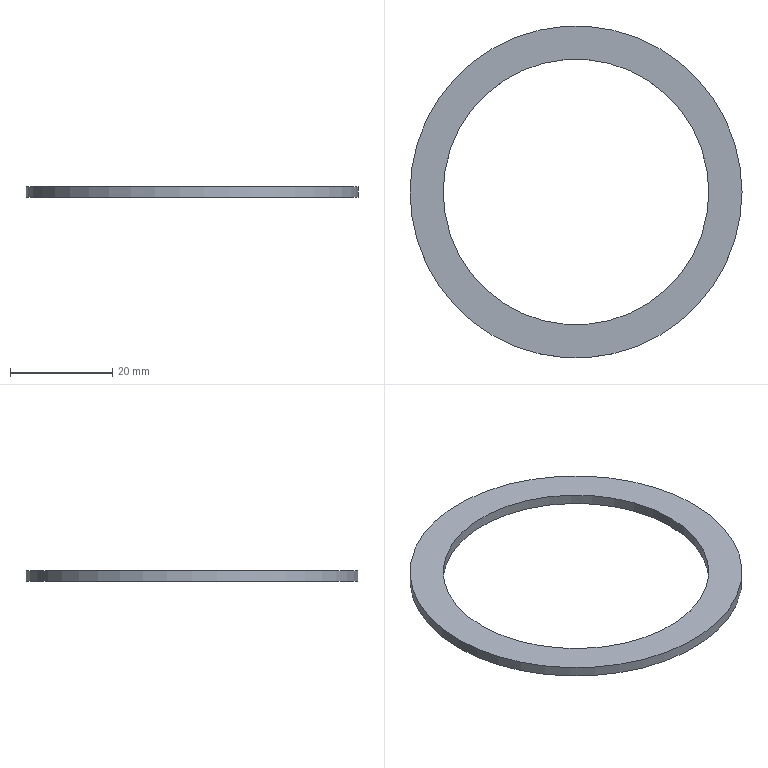Part | NX | features CYLINDER 2, DATUM_CSYS 1 | 1 solid | 4 faces | box 65 x 65 x 2 mm | volume 2389 mm3 | plane 2 | cylinder 2 | commonest cylinder face diameters 52 x1 65 x1
STEP:
#1=CARTESIAN_POINT('',(26.,0.,2.));
#2=VERTEX_POINT('',#1);
#3=CARTESIAN_POINT('',(0.,0.,2.));
#4=DIRECTION('',(0.,0.,-1.));
#5=DIRECTION('',(1.,0.,0.));
#6=AXIS2_PLACEMENT_3D('',#3,#4,#5);
#7=CIRCLE('',#6,26.);
#8=EDGE_CURVE('',#2,#2,#7,.T.);
#9=ORIENTED_EDGE('',*,*,#8,.T.);
#10=EDGE_LOOP('',(#9));
#11=FACE_BOUND('',#10,.T.);
#12=CARTESIAN_POINT('',(32.5,0.,2.));
#13=VERTEX_POINT('',#12);
#14=CARTESIAN_POINT('',(0.,0.,2.));
#15=DIRECTION('',(0.,0.,-1.));
#16=DIRECTION('',(1.,0.,0.));
#17=AXIS2_PLACEMENT_3D('',#14,#15,#16);
#18=CIRCLE('',#17,32.5);
#19=EDGE_CURVE('',#13,#13,#18,.T.);
#20=ORIENTED_EDGE('',*,*,#19,.F.);
#21=EDGE_LOOP('',(#20));
#22=FACE_BOUND('',#21,.T.);
#23=CARTESIAN_POINT('',(0.,0.,2.));
#24=DIRECTION('',(0.,0.,1.));
#25=DIRECTION('',(1.,0.,0.));
#26=AXIS2_PLACEMENT_3D('',#23,#24,#25);
#27=PLANE('',#26);
#28=ADVANCED_FACE('',(#11,#22),#27,.T.);
#29=CARTESIAN_POINT('',(26.,0.,0.));
#30=VERTEX_POINT('',#29);
#31=CARTESIAN_POINT('',(0.,0.,0.));
#32=DIRECTION('',(0.,0.,1.));
#33=DIRECTION('',(1.,0.,0.));
#34=AXIS2_PLACEMENT_3D('',#31,#32,#33);
#35=CIRCLE('',#34,26.);
#36=EDGE_CURVE('',#30,#30,#35,.T.);
#37=ORIENTED_EDGE('',*,*,#36,.T.);
#38=EDGE_LOOP('',(#37));
#39=FACE_BOUND('',#38,.T.);
#40=CARTESIAN_POINT('',(32.5,0.,0.));
#41=VERTEX_POINT('',#40);
#42=CARTESIAN_POINT('',(0.,0.,0.));
#43=DIRECTION('',(0.,0.,1.));
#44=DIRECTION('',(1.,0.,0.));
#45=AXIS2_PLACEMENT_3D('',#42,#43,#44);
#46=CIRCLE('',#45,32.5);
#47=EDGE_CURVE('',#41,#41,#46,.T.);
#48=ORIENTED_EDGE('',*,*,#47,.F.);
#49=EDGE_LOOP('',(#48));
#50=FACE_BOUND('',#49,.T.);
#51=CARTESIAN_POINT('',(0.,0.,0.));
#52=DIRECTION('',(0.,0.,-1.));
#53=DIRECTION('',(-1.,0.,0.));
#54=AXIS2_PLACEMENT_3D('',#51,#52,#53);
#55=PLANE('',#54);
#56=ADVANCED_FACE('',(#39,#50),#55,.T.);
#57=ORIENTED_EDGE('',*,*,#19,.T.);
#58=EDGE_LOOP('',(#57));
#59=FACE_BOUND('',#58,.T.);
#60=ORIENTED_EDGE('',*,*,#47,.T.);
#61=EDGE_LOOP('',(#60));
#62=FACE_BOUND('',#61,.T.);
#63=CARTESIAN_POINT('',(0.,0.,0.));
#64=DIRECTION('',(0.,0.,1.));
#65=DIRECTION('',(1.,0.,0.));
#66=AXIS2_PLACEMENT_3D('',#63,#64,#65);
#67=CYLINDRICAL_SURFACE('',#66,32.5);
#68=ADVANCED_FACE('',(#59,#62),#67,.T.);
#69=ORIENTED_EDGE('',*,*,#8,.F.);
#70=EDGE_LOOP('',(#69));
#71=FACE_BOUND('',#70,.T.);
#72=ORIENTED_EDGE('',*,*,#36,.F.);
#73=EDGE_LOOP('',(#72));
#74=FACE_BOUND('',#73,.T.);
#75=CARTESIAN_POINT('',(0.,0.,0.));
#76=DIRECTION('',(0.,0.,1.));
#77=DIRECTION('',(1.,0.,0.));
#78=AXIS2_PLACEMENT_3D('',#75,#76,#77);
#79=CYLINDRICAL_SURFACE('',#78,26.);
#80=ADVANCED_FACE('',(#71,#74),#79,.F.);
#81=CLOSED_SHELL('',(#28,#56,#68,#80));
#82=MANIFOLD_SOLID_BREP('',#81);
#83=(LENGTH_UNIT()NAMED_UNIT(*)SI_UNIT(.MILLI.,.METRE.));
#84=UNCERTAINTY_MEASURE_WITH_UNIT(LENGTH_MEASURE(0.00001),#83,'','');
#85=(NAMED_UNIT(*)PLANE_ANGLE_UNIT()SI_UNIT($,.RADIAN.));
#86=(NAMED_UNIT(*)SI_UNIT($,.STERADIAN.)SOLID_ANGLE_UNIT());
#87=(GEOMETRIC_REPRESENTATION_CONTEXT(3)GLOBAL_UNCERTAINTY_ASSIGNED_CONTEXT((#84))GLOBAL_UNIT_ASSIGNED_CONTEXT((#83,#85,#86))REPRESENTATION_CONTEXT('',''));
#88=ADVANCED_BREP_SHAPE_REPRESENTATION('',(#82),#87);